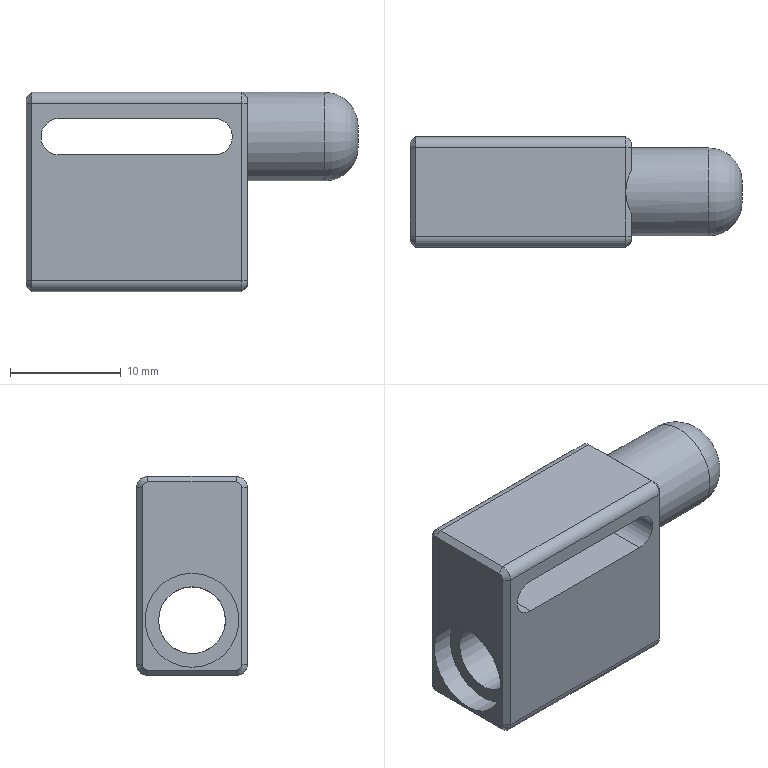Part | NX | 1 solid | 37 faces | box 30 x 10 x 18 mm | volume 2854 mm3 | plane 19 | cylinder 9 | cone 8 | torus 1 | commonest cylinder face diameters 2 x4 3.3 x2 6.05 x1 8 x1 8.5 x1
STEP:
#1=CARTESIAN_POINT('',(5.,9.,3.5));
#2=VERTEX_POINT('',#1);
#3=CARTESIAN_POINT('',(4.5,9.,4.));
#4=VERTEX_POINT('',#3);
#5=CARTESIAN_POINT('',(5.,9.,3.5));
#6=DIRECTION('',(-0.7071,0.,0.7071));
#7=VECTOR('',#6,1000.);
#8=LINE('',#5,#7);
#9=EDGE_CURVE('',#2,#4,#8,.T.);
#10=ORIENTED_EDGE('',*,*,#9,.T.);
#11=CARTESIAN_POINT('',(4.5,5.,4.));
#12=VERTEX_POINT('',#11);
#13=CARTESIAN_POINT('',(4.5,10.,4.));
#14=DIRECTION('',(0.,1.,0.));
#15=VECTOR('',#14,1000.);
#16=LINE('',#13,#15);
#17=EDGE_CURVE('',#12,#4,#16,.T.);
#18=ORIENTED_EDGE('',*,*,#17,.F.);
#19=CARTESIAN_POINT('',(5.,6.936,3.5));
#20=VERTEX_POINT('',#19);
#21=CARTESIAN_POINT('',(8.5,5.,0.));
#22=DIRECTION('',(0.7071,0.,0.7071));
#23=DIRECTION('',(0.7071,0.,-0.7071));
#24=AXIS2_PLACEMENT_3D('',#21,#22,#23);
#25=ELLIPSE('',#24,5.657,4.);
#26=EDGE_CURVE('',#20,#12,#25,.T.);
#27=ORIENTED_EDGE('',*,*,#26,.F.);
#28=CARTESIAN_POINT('',(5.,10.,3.5));
#29=DIRECTION('',(0.,-1.,0.));
#30=VECTOR('',#29,1000.);
#31=LINE('',#28,#30);
#32=EDGE_CURVE('',#2,#20,#31,.T.);
#33=ORIENTED_EDGE('',*,*,#32,.F.);
#34=EDGE_LOOP('',(#10,#18,#27,#33));
#35=FACE_BOUND('',#34,.T.);
#36=CARTESIAN_POINT('',(5.,10.,3.5));
#37=DIRECTION('',(-0.7071,0.,-0.7071));
#38=DIRECTION('',(0.,-1.,0.));
#39=AXIS2_PLACEMENT_3D('',#36,#37,#38);
#40=PLANE('',#39);
#41=ADVANCED_FACE('',(#35),#40,.F.);
#42=CARTESIAN_POINT('',(5.,3.064,3.5));
#43=VERTEX_POINT('',#42);
#44=CARTESIAN_POINT('',(5.,1.,3.5));
#45=VERTEX_POINT('',#44);
#46=CARTESIAN_POINT('',(5.,10.,3.5));
#47=DIRECTION('',(0.,-1.,0.));
#48=VECTOR('',#47,1000.);
#49=LINE('',#46,#48);
#50=EDGE_CURVE('',#43,#45,#49,.T.);
#51=ORIENTED_EDGE('',*,*,#50,.F.);
#52=CARTESIAN_POINT('',(8.5,5.,0.));
#53=DIRECTION('',(0.7071,0.,0.7071));
#54=DIRECTION('',(0.7071,0.,-0.7071));
#55=AXIS2_PLACEMENT_3D('',#52,#53,#54);
#56=ELLIPSE('',#55,5.657,4.);
#57=EDGE_CURVE('',#12,#43,#56,.T.);
#58=ORIENTED_EDGE('',*,*,#57,.F.);
#59=CARTESIAN_POINT('',(4.5,1.,4.));
#60=VERTEX_POINT('',#59);
#61=CARTESIAN_POINT('',(4.5,10.,4.));
#62=DIRECTION('',(0.,1.,0.));
#63=VECTOR('',#62,1000.);
#64=LINE('',#61,#63);
#65=EDGE_CURVE('',#60,#12,#64,.T.);
#66=ORIENTED_EDGE('',*,*,#65,.F.);
#67=CARTESIAN_POINT('',(4.5,1.,4.));
#68=DIRECTION('',(0.7071,0.,-0.7071));
#69=VECTOR('',#68,1000.);
#70=LINE('',#67,#69);
#71=EDGE_CURVE('',#60,#45,#70,.T.);
#72=ORIENTED_EDGE('',*,*,#71,.T.);
#73=EDGE_LOOP('',(#51,#58,#66,#72));
#74=FACE_BOUND('',#73,.T.);
#75=CARTESIAN_POINT('',(5.,10.,3.5));
#76=DIRECTION('',(-0.7071,0.,-0.7071));
#77=DIRECTION('',(0.,-1.,0.));
#78=AXIS2_PLACEMENT_3D('',#75,#76,#77);
#79=PLANE('',#78);
#80=ADVANCED_FACE('',(#74),#79,.F.);
#81=CARTESIAN_POINT('',(5.,9.5,3.));
#82=VERTEX_POINT('',#81);
#83=CARTESIAN_POINT('',(4.5,10.,3.));
#84=VERTEX_POINT('',#83);
#85=CARTESIAN_POINT('',(5.,9.5,3.));
#86=DIRECTION('',(-0.7071,0.7071,0.));
#87=VECTOR('',#86,1000.);
#88=LINE('',#85,#87);
#89=EDGE_CURVE('',#82,#84,#88,.T.);
#90=ORIENTED_EDGE('',*,*,#89,.T.);
#91=CARTESIAN_POINT('',(4.5,9.,3.));
#92=DIRECTION('',(-1.,0.,0.));
#93=DIRECTION('',(0.,0.,1.));
#94=AXIS2_PLACEMENT_3D('',#91,#92,#93);
#95=CIRCLE('',#94,1.);
#96=EDGE_CURVE('',#4,#84,#95,.T.);
#97=ORIENTED_EDGE('',*,*,#96,.F.);
#98=ORIENTED_EDGE('',*,*,#9,.F.);
#99=CARTESIAN_POINT('',(5.,9.,3.));
#100=DIRECTION('',(1.,0.,0.));
#101=DIRECTION('',(0.,-1.,0.));
#102=AXIS2_PLACEMENT_3D('',#99,#100,#101);
#103=CIRCLE('',#102,0.5);
#104=EDGE_CURVE('',#82,#2,#103,.T.);
#105=ORIENTED_EDGE('',*,*,#104,.F.);
#106=EDGE_LOOP('',(#90,#97,#98,#105));
#107=FACE_BOUND('',#106,.T.);
#108=CARTESIAN_POINT('',(5.,9.,3.));
#109=DIRECTION('',(-1.,0.,0.));
#110=DIRECTION('',(0.,0.,1.));
#111=AXIS2_PLACEMENT_3D('',#108,#109,#110);
#112=CONICAL_SURFACE('',#111,0.5,0.7854);
#113=ADVANCED_FACE('',(#107),#112,.T.);
#114=CARTESIAN_POINT('',(4.5,0.,3.));
#115=VERTEX_POINT('',#114);
#116=CARTESIAN_POINT('',(5.,0.5,3.));
#117=VERTEX_POINT('',#116);
#118=CARTESIAN_POINT('',(4.5,0.,3.));
#119=DIRECTION('',(0.7071,0.7071,0.));
#120=VECTOR('',#119,1000.);
#121=LINE('',#118,#120);
#122=EDGE_CURVE('',#115,#117,#121,.T.);
#123=ORIENTED_EDGE('',*,*,#122,.T.);
#124=CARTESIAN_POINT('',(5.,1.,3.));
#125=DIRECTION('',(1.,0.,0.));
#126=DIRECTION('',(0.,-1.,0.));
#127=AXIS2_PLACEMENT_3D('',#124,#125,#126);
#128=CIRCLE('',#127,0.5);
#129=EDGE_CURVE('',#45,#117,#128,.T.);
#130=ORIENTED_EDGE('',*,*,#129,.F.);
#131=ORIENTED_EDGE('',*,*,#71,.F.);
#132=CARTESIAN_POINT('',(4.5,1.,3.));
#133=DIRECTION('',(-1.,0.,0.));
#134=DIRECTION('',(0.,0.,1.));
#135=AXIS2_PLACEMENT_3D('',#132,#133,#134);
#136=CIRCLE('',#135,1.);
#137=EDGE_CURVE('',#115,#60,#136,.T.);
#138=ORIENTED_EDGE('',*,*,#137,.F.);
#139=EDGE_LOOP('',(#123,#130,#131,#138));
#140=FACE_BOUND('',#139,.T.);
#141=CARTESIAN_POINT('',(5.,1.,3.));
#142=DIRECTION('',(-1.,0.,0.));
#143=DIRECTION('',(0.,0.,1.));
#144=AXIS2_PLACEMENT_3D('',#141,#142,#143);
#145=CONICAL_SURFACE('',#144,0.5,0.7854);
#146=ADVANCED_FACE('',(#140),#145,.T.);
#147=CARTESIAN_POINT('',(5.,9.5,-13.));
#148=VERTEX_POINT('',#147);
#149=CARTESIAN_POINT('',(4.5,10.,-13.));
#150=VERTEX_POINT('',#149);
#151=CARTESIAN_POINT('',(5.,9.5,-13.));
#152=DIRECTION('',(-0.7071,0.7071,0.));
#153=VECTOR('',#152,1000.);
#154=LINE('',#151,#153);
#155=EDGE_CURVE('',#148,#150,#154,.T.);
#156=ORIENTED_EDGE('',*,*,#155,.T.);
#157=CARTESIAN_POINT('',(4.5,10.,0.));
#158=DIRECTION('',(0.,0.,-1.));
#159=VECTOR('',#158,1000.);
#160=LINE('',#157,#159);
#161=EDGE_CURVE('',#84,#150,#160,.T.);
#162=ORIENTED_EDGE('',*,*,#161,.F.);
#163=ORIENTED_EDGE('',*,*,#89,.F.);
#164=CARTESIAN_POINT('',(5.,9.5,-14.));
#165=DIRECTION('',(0.,0.,1.));
#166=VECTOR('',#165,1000.);
#167=LINE('',#164,#166);
#168=EDGE_CURVE('',#148,#82,#167,.T.);
#169=ORIENTED_EDGE('',*,*,#168,.F.);
#170=EDGE_LOOP('',(#156,#162,#163,#169));
#171=FACE_BOUND('',#170,.T.);
#172=CARTESIAN_POINT('',(5.,9.5,-14.));
#173=DIRECTION('',(-0.7071,-0.7071,0.));
#174=DIRECTION('',(0.,0.,1.));
#175=AXIS2_PLACEMENT_3D('',#172,#173,#174);
#176=PLANE('',#175);
#177=ADVANCED_FACE('',(#171),#176,.F.);
#178=CARTESIAN_POINT('',(4.5,0.,-13.));
#179=VERTEX_POINT('',#178);
#180=CARTESIAN_POINT('',(5.,0.5,-13.));
#181=VERTEX_POINT('',#180);
#182=CARTESIAN_POINT('',(4.5,0.,-13.));
#183=DIRECTION('',(0.7071,0.7071,0.));
#184=VECTOR('',#183,1000.);
#185=LINE('',#182,#184);
#186=EDGE_CURVE('',#179,#181,#185,.T.);
#187=ORIENTED_EDGE('',*,*,#186,.T.);
#188=CARTESIAN_POINT('',(5.,0.5,-13.));
#189=DIRECTION('',(0.,0.,-1.));
#190=VECTOR('',#189,1000.);
#191=LINE('',#188,#190);
#192=EDGE_CURVE('',#117,#181,#191,.T.);
#193=ORIENTED_EDGE('',*,*,#192,.F.);
#194=ORIENTED_EDGE('',*,*,#122,.F.);
#195=CARTESIAN_POINT('',(4.5,0.,3.));
#196=DIRECTION('',(0.,0.,1.));
#197=VECTOR('',#196,1000.);
#198=LINE('',#195,#197);
#199=EDGE_CURVE('',#179,#115,#198,.T.);
#200=ORIENTED_EDGE('',*,*,#199,.F.);
#201=EDGE_LOOP('',(#187,#193,#194,#200));
#202=FACE_BOUND('',#201,.T.);
#203=CARTESIAN_POINT('',(4.5,0.,0.));
#204=DIRECTION('',(0.7071,-0.7071,0.));
#205=DIRECTION('',(0.,0.,-1.));
#206=AXIS2_PLACEMENT_3D('',#203,#204,#205);
#207=PLANE('',#206);
#208=ADVANCED_FACE('',(#202),#207,.T.);
#209=CARTESIAN_POINT('',(5.,9.,-13.5));
#210=VERTEX_POINT('',#209);
#211=CARTESIAN_POINT('',(4.5,9.,-14.));
#212=VERTEX_POINT('',#211);
#213=CARTESIAN_POINT('',(5.,9.,-13.5));
#214=DIRECTION('',(-0.7071,0.,-0.7071));
#215=VECTOR('',#214,1000.);
#216=LINE('',#213,#215);
#217=EDGE_CURVE('',#210,#212,#216,.T.);
#218=ORIENTED_EDGE('',*,*,#217,.T.);
#219=CARTESIAN_POINT('',(4.5,9.,-13.));
#220=DIRECTION('',(-1.,0.,0.));
#221=DIRECTION('',(0.,0.,1.));
#222=AXIS2_PLACEMENT_3D('',#219,#220,#221);
#223=CIRCLE('',#222,1.);
#224=EDGE_CURVE('',#150,#212,#223,.T.);
#225=ORIENTED_EDGE('',*,*,#224,.F.);
#226=ORIENTED_EDGE('',*,*,#155,.F.);
#227=CARTESIAN_POINT('',(5.,9.,-13.));
#228=DIRECTION('',(1.,0.,0.));
#229=DIRECTION('',(0.,-1.,0.));
#230=AXIS2_PLACEMENT_3D('',#227,#228,#229);
#231=CIRCLE('',#230,0.5);
#232=EDGE_CURVE('',#210,#148,#231,.T.);
#233=ORIENTED_EDGE('',*,*,#232,.F.);
#234=EDGE_LOOP('',(#218,#225,#226,#233));
#235=FACE_BOUND('',#234,.T.);
#236=CARTESIAN_POINT('',(5.,9.,-13.));
#237=DIRECTION('',(-1.,0.,0.));
#238=DIRECTION('',(0.,0.,1.));
#239=AXIS2_PLACEMENT_3D('',#236,#237,#238);
#240=CONICAL_SURFACE('',#239,0.5,0.7854);
#241=ADVANCED_FACE('',(#235),#240,.T.);
#242=CARTESIAN_POINT('',(4.5,1.,-14.));
#243=VERTEX_POINT('',#242);
#244=CARTESIAN_POINT('',(5.,1.,-13.5));
#245=VERTEX_POINT('',#244);
#246=CARTESIAN_POINT('',(4.5,1.,-14.));
#247=DIRECTION('',(0.7071,0.,0.7071));
#248=VECTOR('',#247,1000.);
#249=LINE('',#246,#248);
#250=EDGE_CURVE('',#243,#245,#249,.T.);
#251=ORIENTED_EDGE('',*,*,#250,.T.);
#252=CARTESIAN_POINT('',(5.,1.,-13.));
#253=DIRECTION('',(1.,0.,0.));
#254=DIRECTION('',(0.,-1.,0.));
#255=AXIS2_PLACEMENT_3D('',#252,#253,#254);
#256=CIRCLE('',#255,0.5);
#257=EDGE_CURVE('',#181,#245,#256,.T.);
#258=ORIENTED_EDGE('',*,*,#257,.F.);
#259=ORIENTED_EDGE('',*,*,#186,.F.);
#260=CARTESIAN_POINT('',(4.5,1.,-13.));
#261=DIRECTION('',(-1.,0.,0.));
#262=DIRECTION('',(0.,0.,1.));
#263=AXIS2_PLACEMENT_3D('',#260,#261,#262);
#264=CIRCLE('',#263,1.);
#265=EDGE_CURVE('',#243,#179,#264,.T.);
#266=ORIENTED_EDGE('',*,*,#265,.F.);
#267=EDGE_LOOP('',(#251,#258,#259,#266));
#268=FACE_BOUND('',#267,.T.);
#269=CARTESIAN_POINT('',(5.,1.,-13.));
#270=DIRECTION('',(-1.,0.,0.));
#271=DIRECTION('',(0.,0.,1.));
#272=AXIS2_PLACEMENT_3D('',#269,#270,#271);
#273=CONICAL_SURFACE('',#272,0.5,0.7854);
#274=ADVANCED_FACE('',(#268),#273,.T.);
#275=ORIENTED_EDGE('',*,*,#217,.F.);
#276=CARTESIAN_POINT('',(5.,10.,-13.5));
#277=DIRECTION('',(0.,1.,0.));
#278=VECTOR('',#277,1000.);
#279=LINE('',#276,#278);
#280=EDGE_CURVE('',#245,#210,#279,.T.);
#281=ORIENTED_EDGE('',*,*,#280,.F.);
#282=ORIENTED_EDGE('',*,*,#250,.F.);
#283=CARTESIAN_POINT('',(4.5,0.,-14.));
#284=DIRECTION('',(0.,-1.,0.));
#285=VECTOR('',#284,1000.);
#286=LINE('',#283,#285);
#287=EDGE_CURVE('',#212,#243,#286,.T.);
#288=ORIENTED_EDGE('',*,*,#287,.F.);
#289=EDGE_LOOP('',(#275,#281,#282,#288));
#290=FACE_BOUND('',#289,.T.);
#291=CARTESIAN_POINT('',(4.5,0.,-14.));
#292=DIRECTION('',(-0.7071,0.,0.7071));
#293=DIRECTION('',(0.,-1.,0.));
#294=AXIS2_PLACEMENT_3D('',#291,#292,#293);
#295=PLANE('',#294);
#296=ADVANCED_FACE('',(#290),#295,.F.);
#297=CARTESIAN_POINT('',(-14.5,1.,-14.));
#298=VERTEX_POINT('',#297);
#299=CARTESIAN_POINT('',(-15.,1.,-13.5));
#300=VERTEX_POINT('',#299);
#301=CARTESIAN_POINT('',(-14.5,1.,-14.));
#302=DIRECTION('',(-0.7071,0.,0.7071));
#303=VECTOR('',#302,1000.);
#304=LINE('',#301,#303);
#305=EDGE_CURVE('',#298,#300,#304,.T.);
#306=ORIENTED_EDGE('',*,*,#305,.T.);
#307=CARTESIAN_POINT('',(-15.,9.,-13.5));
#308=VERTEX_POINT('',#307);
#309=CARTESIAN_POINT('',(-15.,10.,-13.5));
#310=DIRECTION('',(0.,-1.,0.));
#311=VECTOR('',#310,1000.);
#312=LINE('',#309,#311);
#313=EDGE_CURVE('',#308,#300,#312,.T.);
#314=ORIENTED_EDGE('',*,*,#313,.F.);
#315=CARTESIAN_POINT('',(-14.5,9.,-14.));
#316=VERTEX_POINT('',#315);
#317=CARTESIAN_POINT('',(-15.,9.,-13.5));
#318=DIRECTION('',(0.7071,0.,-0.7071));
#319=VECTOR('',#318,1000.);
#320=LINE('',#317,#319);
#321=EDGE_CURVE('',#308,#316,#320,.T.);
#322=ORIENTED_EDGE('',*,*,#321,.T.);
#323=CARTESIAN_POINT('',(-14.5,0.,-14.));
#324=DIRECTION('',(0.,1.,0.));
#325=VECTOR('',#324,1000.);
#326=LINE('',#323,#325);
#327=EDGE_CURVE('',#298,#316,#326,.T.);
#328=ORIENTED_EDGE('',*,*,#327,.F.);
#329=EDGE_LOOP('',(#306,#314,#322,#328));
#330=FACE_BOUND('',#329,.T.);
#331=CARTESIAN_POINT('',(-14.5,0.,-14.));
#332=DIRECTION('',(0.7071,0.,0.7071));
#333=DIRECTION('',(0.,1.,0.));
#334=AXIS2_PLACEMENT_3D('',#331,#332,#333);
#335=PLANE('',#334);
#336=ADVANCED_FACE('',(#330),#335,.F.);
#337=CARTESIAN_POINT('',(-15.,9.5,-13.));
#338=VERTEX_POINT('',#337);
#339=CARTESIAN_POINT('',(-14.5,10.,-13.));
#340=VERTEX_POINT('',#339);
#341=CARTESIAN_POINT('',(-15.,9.5,-13.));
#342=DIRECTION('',(0.7071,0.7071,0.));
#343=VECTOR('',#342,1000.);
#344=LINE('',#341,#343);
#345=EDGE_CURVE('',#338,#340,#344,.T.);
#346=ORIENTED_EDGE('',*,*,#345,.T.);
#347=CARTESIAN_POINT('',(-14.5,9.,-13.));
#348=DIRECTION('',(1.,0.,0.));
#349=DIRECTION('',(0.,0.,-1.));
#350=AXIS2_PLACEMENT_3D('',#347,#348,#349);
#351=CIRCLE('',#350,1.);
#352=EDGE_CURVE('',#316,#340,#351,.T.);
#353=ORIENTED_EDGE('',*,*,#352,.F.);
#354=ORIENTED_EDGE('',*,*,#321,.F.);
#355=CARTESIAN_POINT('',(-15.,9.,-13.));
#356=DIRECTION('',(-1.,0.,0.));
#357=DIRECTION('',(0.,0.,-1.));
#358=AXIS2_PLACEMENT_3D('',#355,#356,#357);
#359=CIRCLE('',#358,0.5);
#360=EDGE_CURVE('',#338,#308,#359,.T.);
#361=ORIENTED_EDGE('',*,*,#360,.F.);
#362=EDGE_LOOP('',(#346,#353,#354,#361));
#363=FACE_BOUND('',#362,.T.);
#364=CARTESIAN_POINT('',(-15.,9.,-13.));
#365=DIRECTION('',(1.,0.,0.));
#366=DIRECTION('',(0.,0.,-1.));
#367=AXIS2_PLACEMENT_3D('',#364,#365,#366);
#368=CONICAL_SURFACE('',#367,0.5,0.7854);
#369=ADVANCED_FACE('',(#363),#368,.T.);
#370=CARTESIAN_POINT('',(-14.5,0.,-13.));
#371=VERTEX_POINT('',#370);
#372=CARTESIAN_POINT('',(-15.,0.5,-13.));
#373=VERTEX_POINT('',#372);
#374=CARTESIAN_POINT('',(-14.5,0.,-13.));
#375=DIRECTION('',(-0.7071,0.7071,0.));
#376=VECTOR('',#375,1000.);
#377=LINE('',#374,#376);
#378=EDGE_CURVE('',#371,#373,#377,.T.);
#379=ORIENTED_EDGE('',*,*,#378,.T.);
#380=CARTESIAN_POINT('',(-15.,1.,-13.));
#381=DIRECTION('',(-1.,0.,0.));
#382=DIRECTION('',(0.,0.,-1.));
#383=AXIS2_PLACEMENT_3D('',#380,#381,#382);
#384=CIRCLE('',#383,0.5);
#385=EDGE_CURVE('',#300,#373,#384,.T.);
#386=ORIENTED_EDGE('',*,*,#385,.F.);
#387=ORIENTED_EDGE('',*,*,#305,.F.);
#388=CARTESIAN_POINT('',(-14.5,1.,-13.));
#389=DIRECTION('',(1.,0.,0.));
#390=DIRECTION('',(0.,0.,-1.));
#391=AXIS2_PLACEMENT_3D('',#388,#389,#390);
#392=CIRCLE('',#391,1.);
#393=EDGE_CURVE('',#371,#298,#392,.T.);
#394=ORIENTED_EDGE('',*,*,#393,.F.);
#395=EDGE_LOOP('',(#379,#386,#387,#394));
#396=FACE_BOUND('',#395,.T.);
#397=CARTESIAN_POINT('',(-15.,1.,-13.));
#398=DIRECTION('',(1.,0.,0.));
#399=DIRECTION('',(0.,0.,-1.));
#400=AXIS2_PLACEMENT_3D('',#397,#398,#399);
#401=CONICAL_SURFACE('',#400,0.5,0.7854);
#402=ADVANCED_FACE('',(#396),#401,.T.);
#403=CARTESIAN_POINT('',(-15.,9.5,3.));
#404=VERTEX_POINT('',#403);
#405=CARTESIAN_POINT('',(-14.5,10.,3.));
#406=VERTEX_POINT('',#405);
#407=CARTESIAN_POINT('',(-15.,9.5,3.));
#408=DIRECTION('',(0.7071,0.7071,0.));
#409=VECTOR('',#408,1000.);
#410=LINE('',#407,#409);
#411=EDGE_CURVE('',#404,#406,#410,.T.);
#412=ORIENTED_EDGE('',*,*,#411,.T.);
#413=CARTESIAN_POINT('',(-14.5,10.,0.));
#414=DIRECTION('',(0.,0.,1.));
#415=VECTOR('',#414,1000.);
#416=LINE('',#413,#415);
#417=EDGE_CURVE('',#340,#406,#416,.T.);
#418=ORIENTED_EDGE('',*,*,#417,.F.);
#419=ORIENTED_EDGE('',*,*,#345,.F.);
#420=CARTESIAN_POINT('',(-15.,9.5,4.));
#421=DIRECTION('',(0.,0.,-1.));
#422=VECTOR('',#421,1000.);
#423=LINE('',#420,#422);
#424=EDGE_CURVE('',#404,#338,#423,.T.);
#425=ORIENTED_EDGE('',*,*,#424,.F.);
#426=EDGE_LOOP('',(#412,#418,#419,#425));
#427=FACE_BOUND('',#426,.T.);
#428=CARTESIAN_POINT('',(-14.5,10.,0.));
#429=DIRECTION('',(0.7071,-0.7071,0.));
#430=DIRECTION('',(0.,0.,1.));
#431=AXIS2_PLACEMENT_3D('',#428,#429,#430);
#432=PLANE('',#431);
#433=ADVANCED_FACE('',(#427),#432,.F.);
#434=CARTESIAN_POINT('',(-14.5,0.,3.));
#435=VERTEX_POINT('',#434);
#436=CARTESIAN_POINT('',(-15.,0.5,3.));
#437=VERTEX_POINT('',#436);
#438=CARTESIAN_POINT('',(-14.5,0.,3.));
#439=DIRECTION('',(-0.7071,0.7071,0.));
#440=VECTOR('',#439,1000.);
#441=LINE('',#438,#440);
#442=EDGE_CURVE('',#435,#437,#441,.T.);
#443=ORIENTED_EDGE('',*,*,#442,.T.);
#444=CARTESIAN_POINT('',(-15.,0.5,3.));
#445=DIRECTION('',(0.,0.,1.));
#446=VECTOR('',#445,1000.);
#447=LINE('',#444,#446);
#448=EDGE_CURVE('',#373,#437,#447,.T.);
#449=ORIENTED_EDGE('',*,*,#448,.F.);
#450=ORIENTED_EDGE('',*,*,#378,.F.);
#451=CARTESIAN_POINT('',(-14.5,0.,-13.));
#452=DIRECTION('',(0.,0.,-1.));
#453=VECTOR('',#452,1000.);
#454=LINE('',#451,#453);
#455=EDGE_CURVE('',#435,#371,#454,.T.);
#456=ORIENTED_EDGE('',*,*,#455,.F.);
#457=EDGE_LOOP('',(#443,#449,#450,#456));
#458=FACE_BOUND('',#457,.T.);
#459=CARTESIAN_POINT('',(-15.,0.5,4.));
#460=DIRECTION('',(-0.7071,-0.7071,0.));
#461=DIRECTION('',(0.,0.,-1.));
#462=AXIS2_PLACEMENT_3D('',#459,#460,#461);
#463=PLANE('',#462);
#464=ADVANCED_FACE('',(#458),#463,.T.);
#465=CARTESIAN_POINT('',(-15.,9.,3.5));
#466=VERTEX_POINT('',#465);
#467=CARTESIAN_POINT('',(-14.5,9.,4.));
#468=VERTEX_POINT('',#467);
#469=CARTESIAN_POINT('',(-15.,9.,3.5));
#470=DIRECTION('',(0.7071,0.,0.7071));
#471=VECTOR('',#470,1000.);
#472=LINE('',#469,#471);
#473=EDGE_CURVE('',#466,#468,#472,.T.);
#474=ORIENTED_EDGE('',*,*,#473,.T.);
#475=CARTESIAN_POINT('',(-14.5,9.,3.));
#476=DIRECTION('',(1.,0.,0.));
#477=DIRECTION('',(0.,0.,-1.));
#478=AXIS2_PLACEMENT_3D('',#475,#476,#477);
#479=CIRCLE('',#478,1.);
#480=EDGE_CURVE('',#406,#468,#479,.T.);
#481=ORIENTED_EDGE('',*,*,#480,.F.);
#482=ORIENTED_EDGE('',*,*,#411,.F.);
#483=CARTESIAN_POINT('',(-15.,9.,3.));
#484=DIRECTION('',(-1.,0.,0.));
#485=DIRECTION('',(0.,0.,-1.));
#486=AXIS2_PLACEMENT_3D('',#483,#484,#485);
#487=CIRCLE('',#486,0.5);
#488=EDGE_CURVE('',#466,#404,#487,.T.);
#489=ORIENTED_EDGE('',*,*,#488,.F.);
#490=EDGE_LOOP('',(#474,#481,#482,#489));
#491=FACE_BOUND('',#490,.T.);
#492=CARTESIAN_POINT('',(-15.,9.,3.));
#493=DIRECTION('',(1.,0.,0.));
#494=DIRECTION('',(0.,0.,-1.));
#495=AXIS2_PLACEMENT_3D('',#492,#493,#494);
#496=CONICAL_SURFACE('',#495,0.5,0.7854);
#497=ADVANCED_FACE('',(#491),#496,.T.);
#498=CARTESIAN_POINT('',(-14.5,1.,4.));
#499=VERTEX_POINT('',#498);
#500=CARTESIAN_POINT('',(-15.,1.,3.5));
#501=VERTEX_POINT('',#500);
#502=CARTESIAN_POINT('',(-14.5,1.,4.));
#503=DIRECTION('',(-0.7071,0.,-0.7071));
#504=VECTOR('',#503,1000.);
#505=LINE('',#502,#504);
#506=EDGE_CURVE('',#499,#501,#505,.T.);
#507=ORIENTED_EDGE('',*,*,#506,.T.);
#508=CARTESIAN_POINT('',(-15.,1.,3.));
#509=DIRECTION('',(-1.,0.,0.));
#510=DIRECTION('',(0.,0.,-1.));
#511=AXIS2_PLACEMENT_3D('',#508,#509,#510);
#512=CIRCLE('',#511,0.5);
#513=EDGE_CURVE('',#437,#501,#512,.T.);
#514=ORIENTED_EDGE('',*,*,#513,.F.);
#515=ORIENTED_EDGE('',*,*,#442,.F.);
#516=CARTESIAN_POINT('',(-14.5,1.,3.));
#517=DIRECTION('',(1.,0.,0.));
#518=DIRECTION('',(0.,0.,-1.));
#519=AXIS2_PLACEMENT_3D('',#516,#517,#518);
#520=CIRCLE('',#519,1.);
#521=EDGE_CURVE('',#499,#435,#520,.T.);
#522=ORIENTED_EDGE('',*,*,#521,.F.);
#523=EDGE_LOOP('',(#507,#514,#515,#522));
#524=FACE_BOUND('',#523,.T.);
#525=CARTESIAN_POINT('',(-15.,1.,3.));
#526=DIRECTION('',(1.,0.,0.));
#527=DIRECTION('',(0.,0.,-1.));
#528=AXIS2_PLACEMENT_3D('',#525,#526,#527);
#529=CONICAL_SURFACE('',#528,0.5,0.7854);
#530=ADVANCED_FACE('',(#524),#529,.T.);
#531=ORIENTED_EDGE('',*,*,#473,.F.);
#532=CARTESIAN_POINT('',(-15.,10.,3.5));
#533=DIRECTION('',(0.,1.,0.));
#534=VECTOR('',#533,1000.);
#535=LINE('',#532,#534);
#536=EDGE_CURVE('',#501,#466,#535,.T.);
#537=ORIENTED_EDGE('',*,*,#536,.F.);
#538=ORIENTED_EDGE('',*,*,#506,.F.);
#539=CARTESIAN_POINT('',(-14.5,10.,4.));
#540=DIRECTION('',(0.,-1.,0.));
#541=VECTOR('',#540,1000.);
#542=LINE('',#539,#541);
#543=EDGE_CURVE('',#468,#499,#542,.T.);
#544=ORIENTED_EDGE('',*,*,#543,.F.);
#545=EDGE_LOOP('',(#531,#537,#538,#544));
#546=FACE_BOUND('',#545,.T.);
#547=CARTESIAN_POINT('',(-14.5,10.,4.));
#548=DIRECTION('',(0.7071,0.,-0.7071));
#549=DIRECTION('',(0.,-1.,0.));
#550=AXIS2_PLACEMENT_3D('',#547,#548,#549);
#551=PLANE('',#550);
#552=ADVANCED_FACE('',(#546),#551,.F.);
#553=CARTESIAN_POINT('',(-13.,5.,-5.975));
#554=VERTEX_POINT('',#553);
#555=CARTESIAN_POINT('',(-13.,5.,-9.));
#556=DIRECTION('',(1.,0.,0.));
#557=DIRECTION('',(0.,0.,1.));
#558=AXIS2_PLACEMENT_3D('',#555,#556,#557);
#559=CIRCLE('',#558,3.025);
#560=EDGE_CURVE('',#554,#554,#559,.T.);
#561=ORIENTED_EDGE('',*,*,#560,.T.);
#562=EDGE_LOOP('',(#561));
#563=FACE_BOUND('',#562,.T.);
#564=CARTESIAN_POINT('',(-13.,5.,-4.75));
#565=VERTEX_POINT('',#564);
#566=CARTESIAN_POINT('',(-13.,5.,-9.));
#567=DIRECTION('',(-1.,0.,0.));
#568=DIRECTION('',(0.,0.,1.));
#569=AXIS2_PLACEMENT_3D('',#566,#567,#568);
#570=CIRCLE('',#569,4.25);
#571=EDGE_CURVE('',#565,#565,#570,.T.);
#572=ORIENTED_EDGE('',*,*,#571,.T.);
#573=EDGE_LOOP('',(#572));
#574=FACE_BOUND('',#573,.T.);
#575=CARTESIAN_POINT('',(-13.,5.,-9.));
#576=DIRECTION('',(-1.,0.,0.));
#577=DIRECTION('',(0.,0.,1.));
#578=AXIS2_PLACEMENT_3D('',#575,#576,#577);
#579=PLANE('',#578);
#580=ADVANCED_FACE('',(#563,#574),#579,.T.);
#581=CARTESIAN_POINT('',(5.,1.,4.));
#582=DIRECTION('',(1.,0.,0.));
#583=VECTOR('',#582,1000.);
#584=LINE('',#581,#583);
#585=EDGE_CURVE('',#499,#60,#584,.T.);
#586=ORIENTED_EDGE('',*,*,#585,.F.);
#587=ORIENTED_EDGE('',*,*,#521,.T.);
#588=CARTESIAN_POINT('',(-15.,0.,3.));
#589=DIRECTION('',(-1.,0.,0.));
#590=VECTOR('',#589,1000.);
#591=LINE('',#588,#590);
#592=EDGE_CURVE('',#115,#435,#591,.T.);
#593=ORIENTED_EDGE('',*,*,#592,.F.);
#594=ORIENTED_EDGE('',*,*,#137,.T.);
#595=EDGE_LOOP('',(#586,#587,#593,#594));
#596=FACE_BOUND('',#595,.T.);
#597=CARTESIAN_POINT('',(-15.,1.,3.));
#598=DIRECTION('',(-1.,0.,0.));
#599=DIRECTION('',(0.,0.,1.));
#600=AXIS2_PLACEMENT_3D('',#597,#598,#599);
#601=CYLINDRICAL_SURFACE('',#600,1.);
#602=ADVANCED_FACE('',(#596),#601,.T.);
#603=CARTESIAN_POINT('',(0.,10.,3.));
#604=DIRECTION('',(1.,0.,0.));
#605=VECTOR('',#604,1000.);
#606=LINE('',#603,#605);
#607=EDGE_CURVE('',#406,#84,#606,.T.);
#608=ORIENTED_EDGE('',*,*,#607,.F.);
#609=ORIENTED_EDGE('',*,*,#480,.T.);
#610=CARTESIAN_POINT('',(-15.,9.,4.));
#611=DIRECTION('',(-1.,0.,0.));
#612=VECTOR('',#611,1000.);
#613=LINE('',#610,#612);
#614=EDGE_CURVE('',#4,#468,#613,.T.);
#615=ORIENTED_EDGE('',*,*,#614,.F.);
#616=ORIENTED_EDGE('',*,*,#96,.T.);
#617=EDGE_LOOP('',(#608,#609,#615,#616));
#618=FACE_BOUND('',#617,.T.);
#619=CARTESIAN_POINT('',(0.,9.,3.));
#620=DIRECTION('',(1.,0.,0.));
#621=DIRECTION('',(0.,0.,-1.));
#622=AXIS2_PLACEMENT_3D('',#619,#620,#621);
#623=CYLINDRICAL_SURFACE('',#622,1.);
#624=ADVANCED_FACE('',(#618),#623,.T.);
#625=CARTESIAN_POINT('',(5.,0.,-13.));
#626=DIRECTION('',(1.,0.,0.));
#627=VECTOR('',#626,1000.);
#628=LINE('',#625,#627);
#629=EDGE_CURVE('',#371,#179,#628,.T.);
#630=ORIENTED_EDGE('',*,*,#629,.F.);
#631=ORIENTED_EDGE('',*,*,#393,.T.);
#632=CARTESIAN_POINT('',(-15.,1.,-14.));
#633=DIRECTION('',(-1.,0.,0.));
#634=VECTOR('',#633,1000.);
#635=LINE('',#632,#634);
#636=EDGE_CURVE('',#243,#298,#635,.T.);
#637=ORIENTED_EDGE('',*,*,#636,.F.);
#638=ORIENTED_EDGE('',*,*,#265,.T.);
#639=EDGE_LOOP('',(#630,#631,#637,#638));
#640=FACE_BOUND('',#639,.T.);
#641=CARTESIAN_POINT('',(0.,1.,-13.));
#642=DIRECTION('',(1.,0.,0.));
#643=DIRECTION('',(0.,0.,-1.));
#644=AXIS2_PLACEMENT_3D('',#641,#642,#643);
#645=CYLINDRICAL_SURFACE('',#644,1.);
#646=ADVANCED_FACE('',(#640),#645,.T.);
#647=CARTESIAN_POINT('',(0.,9.,-14.));
#648=DIRECTION('',(1.,0.,0.));
#649=VECTOR('',#648,1000.);
#650=LINE('',#647,#649);
#651=EDGE_CURVE('',#316,#212,#650,.T.);
#652=ORIENTED_EDGE('',*,*,#651,.F.);
#653=ORIENTED_EDGE('',*,*,#352,.T.);
#654=CARTESIAN_POINT('',(0.,10.,-13.));
#655=DIRECTION('',(-1.,0.,0.));
#656=VECTOR('',#655,1000.);
#657=LINE('',#654,#656);
#658=EDGE_CURVE('',#150,#340,#657,.T.);
#659=ORIENTED_EDGE('',*,*,#658,.F.);
#660=ORIENTED_EDGE('',*,*,#224,.T.);
#661=EDGE_LOOP('',(#652,#653,#659,#660));
#662=FACE_BOUND('',#661,.T.);
#663=CARTESIAN_POINT('',(0.,9.,-13.));
#664=DIRECTION('',(1.,0.,0.));
#665=DIRECTION('',(0.,0.,-1.));
#666=AXIS2_PLACEMENT_3D('',#663,#664,#665);
#667=CYLINDRICAL_SURFACE('',#666,1.);
#668=ADVANCED_FACE('',(#662),#667,.T.);
#669=ORIENTED_EDGE('',*,*,#636,.T.);
#670=ORIENTED_EDGE('',*,*,#327,.T.);
#671=ORIENTED_EDGE('',*,*,#651,.T.);
#672=ORIENTED_EDGE('',*,*,#287,.T.);
#673=EDGE_LOOP('',(#669,#670,#671,#672));
#674=FACE_BOUND('',#673,.T.);
#675=CARTESIAN_POINT('',(0.,0.,-14.));
#676=DIRECTION('',(0.,0.,1.));
#677=DIRECTION('',(1.,0.,0.));
#678=AXIS2_PLACEMENT_3D('',#675,#676,#677);
#679=PLANE('',#678);
#680=ADVANCED_FACE('',(#674),#679,.F.);
#681=ORIENTED_EDGE('',*,*,#104,.T.);
#682=ORIENTED_EDGE('',*,*,#32,.T.);
#683=CARTESIAN_POINT('',(5.,5.,0.));
#684=DIRECTION('',(1.,0.,0.));
#685=DIRECTION('',(0.,-1.,0.));
#686=AXIS2_PLACEMENT_3D('',#683,#684,#685);
#687=CIRCLE('',#686,4.);
#688=EDGE_CURVE('',#43,#20,#687,.T.);
#689=ORIENTED_EDGE('',*,*,#688,.F.);
#690=ORIENTED_EDGE('',*,*,#50,.T.);
#691=ORIENTED_EDGE('',*,*,#129,.T.);
#692=ORIENTED_EDGE('',*,*,#192,.T.);
#693=ORIENTED_EDGE('',*,*,#257,.T.);
#694=ORIENTED_EDGE('',*,*,#280,.T.);
#695=ORIENTED_EDGE('',*,*,#232,.T.);
#696=ORIENTED_EDGE('',*,*,#168,.T.);
#697=EDGE_LOOP('',(#681,#682,#689,#690,#691,#692,#693,#694,#695,#696));
#698=FACE_BOUND('',#697,.T.);
#699=CARTESIAN_POINT('',(5.,8.025,-9.));
#700=VERTEX_POINT('',#699);
#701=CARTESIAN_POINT('',(5.,5.,-9.));
#702=DIRECTION('',(1.,0.,0.));
#703=DIRECTION('',(0.,1.,0.));
#704=AXIS2_PLACEMENT_3D('',#701,#702,#703);
#705=CIRCLE('',#704,3.025);
#706=EDGE_CURVE('',#700,#700,#705,.T.);
#707=ORIENTED_EDGE('',*,*,#706,.F.);
#708=EDGE_LOOP('',(#707));
#709=FACE_BOUND('',#708,.T.);
#710=CARTESIAN_POINT('',(5.,10.,-14.));
#711=DIRECTION('',(-1.,0.,0.));
#712=DIRECTION('',(0.,-1.,0.));
#713=AXIS2_PLACEMENT_3D('',#710,#711,#712);
#714=PLANE('',#713);
#715=ADVANCED_FACE('',(#698,#709),#714,.F.);
#716=CARTESIAN_POINT('',(2.,0.,1.65));
#717=VERTEX_POINT('',#716);
#718=CARTESIAN_POINT('',(-12.,0.,1.65));
#719=VERTEX_POINT('',#718);
#720=CARTESIAN_POINT('',(0.,0.,1.65));
#721=DIRECTION('',(-1.,0.,0.));
#722=VECTOR('',#721,1000.);
#723=LINE('',#720,#722);
#724=EDGE_CURVE('',#717,#719,#723,.T.);
#725=ORIENTED_EDGE('',*,*,#724,.T.);
#726=CARTESIAN_POINT('',(-12.,10.,1.65));
#727=VERTEX_POINT('',#726);
#728=CARTESIAN_POINT('',(-12.,-101.,1.65));
#729=DIRECTION('',(0.,1.,0.));
#730=VECTOR('',#729,1000.);
#731=LINE('',#728,#730);
#732=EDGE_CURVE('',#719,#727,#731,.T.);
#733=ORIENTED_EDGE('',*,*,#732,.T.);
#734=CARTESIAN_POINT('',(2.,10.,1.65));
#735=VERTEX_POINT('',#734);
#736=CARTESIAN_POINT('',(-12.,10.,1.65));
#737=DIRECTION('',(1.,0.,0.));
#738=VECTOR('',#737,1000.);
#739=LINE('',#736,#738);
#740=EDGE_CURVE('',#727,#735,#739,.T.);
#741=ORIENTED_EDGE('',*,*,#740,.T.);
#742=CARTESIAN_POINT('',(2.,-101.,1.65));
#743=DIRECTION('',(0.,1.,0.));
#744=VECTOR('',#743,1000.);
#745=LINE('',#742,#744);
#746=EDGE_CURVE('',#717,#735,#745,.T.);
#747=ORIENTED_EDGE('',*,*,#746,.F.);
#748=EDGE_LOOP('',(#725,#733,#741,#747));
#749=FACE_BOUND('',#748,.T.);
#750=CARTESIAN_POINT('',(-12.,-101.,1.65));
#751=DIRECTION('',(0.,0.,1.));
#752=DIRECTION('',(1.,0.,0.));
#753=AXIS2_PLACEMENT_3D('',#750,#751,#752);
#754=PLANE('',#753);
#755=ADVANCED_FACE('',(#749),#754,.F.);
#756=CARTESIAN_POINT('',(2.,0.,-1.65));
#757=VERTEX_POINT('',#756);
#758=CARTESIAN_POINT('',(2.,0.,0.));
#759=DIRECTION('',(0.,-1.,0.));
#760=DIRECTION('',(0.,0.,-1.));
#761=AXIS2_PLACEMENT_3D('',#758,#759,#760);
#762=CIRCLE('',#761,1.65);
#763=EDGE_CURVE('',#757,#717,#762,.T.);
#764=ORIENTED_EDGE('',*,*,#763,.T.);
#765=ORIENTED_EDGE('',*,*,#746,.T.);
#766=CARTESIAN_POINT('',(2.,10.,-1.65));
#767=VERTEX_POINT('',#766);
#768=CARTESIAN_POINT('',(2.,10.,0.));
#769=DIRECTION('',(0.,1.,0.));
#770=DIRECTION('',(0.,0.,1.));
#771=AXIS2_PLACEMENT_3D('',#768,#769,#770);
#772=CIRCLE('',#771,1.65);
#773=EDGE_CURVE('',#735,#767,#772,.T.);
#774=ORIENTED_EDGE('',*,*,#773,.T.);
#775=CARTESIAN_POINT('',(2.,-101.,-1.65));
#776=DIRECTION('',(0.,1.,0.));
#777=VECTOR('',#776,1000.);
#778=LINE('',#775,#777);
#779=EDGE_CURVE('',#757,#767,#778,.T.);
#780=ORIENTED_EDGE('',*,*,#779,.F.);
#781=EDGE_LOOP('',(#764,#765,#774,#780));
#782=FACE_BOUND('',#781,.T.);
#783=CARTESIAN_POINT('',(2.,-101.,0.));
#784=DIRECTION('',(0.,1.,0.));
#785=DIRECTION('',(0.,0.,1.));
#786=AXIS2_PLACEMENT_3D('',#783,#784,#785);
#787=CYLINDRICAL_SURFACE('',#786,1.65);
#788=ADVANCED_FACE('',(#782),#787,.F.);
#789=CARTESIAN_POINT('',(-12.,0.,-1.65));
#790=VERTEX_POINT('',#789);
#791=CARTESIAN_POINT('',(0.,0.,-1.65));
#792=DIRECTION('',(1.,0.,0.));
#793=VECTOR('',#792,1000.);
#794=LINE('',#791,#793);
#795=EDGE_CURVE('',#790,#757,#794,.T.);
#796=ORIENTED_EDGE('',*,*,#795,.T.);
#797=ORIENTED_EDGE('',*,*,#779,.T.);
#798=CARTESIAN_POINT('',(-12.,10.,-1.65));
#799=VERTEX_POINT('',#798);
#800=CARTESIAN_POINT('',(-12.,10.,-1.65));
#801=DIRECTION('',(-1.,0.,0.));
#802=VECTOR('',#801,1000.);
#803=LINE('',#800,#802);
#804=EDGE_CURVE('',#767,#799,#803,.T.);
#805=ORIENTED_EDGE('',*,*,#804,.T.);
#806=CARTESIAN_POINT('',(-12.,-101.,-1.65));
#807=DIRECTION('',(0.,1.,0.));
#808=VECTOR('',#807,1000.);
#809=LINE('',#806,#808);
#810=EDGE_CURVE('',#790,#799,#809,.T.);
#811=ORIENTED_EDGE('',*,*,#810,.F.);
#812=EDGE_LOOP('',(#796,#797,#805,#811));
#813=FACE_BOUND('',#812,.T.);
#814=CARTESIAN_POINT('',(-12.,-101.,-1.65));
#815=DIRECTION('',(0.,0.,-1.));
#816=DIRECTION('',(-1.,0.,0.));
#817=AXIS2_PLACEMENT_3D('',#814,#815,#816);
#818=PLANE('',#817);
#819=ADVANCED_FACE('',(#813),#818,.F.);
#820=CARTESIAN_POINT('',(-12.,0.,0.));
#821=DIRECTION('',(0.,-1.,0.));
#822=DIRECTION('',(0.,0.,-1.));
#823=AXIS2_PLACEMENT_3D('',#820,#821,#822);
#824=CIRCLE('',#823,1.65);
#825=EDGE_CURVE('',#719,#790,#824,.T.);
#826=ORIENTED_EDGE('',*,*,#825,.T.);
#827=ORIENTED_EDGE('',*,*,#810,.T.);
#828=CARTESIAN_POINT('',(-12.,10.,0.));
#829=DIRECTION('',(0.,1.,0.));
#830=DIRECTION('',(0.,0.,1.));
#831=AXIS2_PLACEMENT_3D('',#828,#829,#830);
#832=CIRCLE('',#831,1.65);
#833=EDGE_CURVE('',#799,#727,#832,.T.);
#834=ORIENTED_EDGE('',*,*,#833,.T.);
#835=ORIENTED_EDGE('',*,*,#732,.F.);
#836=EDGE_LOOP('',(#826,#827,#834,#835));
#837=FACE_BOUND('',#836,.T.);
#838=CARTESIAN_POINT('',(-12.,-101.,0.));
#839=DIRECTION('',(0.,1.,0.));
#840=DIRECTION('',(0.,0.,1.));
#841=AXIS2_PLACEMENT_3D('',#838,#839,#840);
#842=CYLINDRICAL_SURFACE('',#841,1.65);
#843=ADVANCED_FACE('',(#837),#842,.F.);
#844=ORIENTED_EDGE('',*,*,#825,.F.);
#845=ORIENTED_EDGE('',*,*,#724,.F.);
#846=ORIENTED_EDGE('',*,*,#763,.F.);
#847=ORIENTED_EDGE('',*,*,#795,.F.);
#848=EDGE_LOOP('',(#844,#845,#846,#847));
#849=FACE_BOUND('',#848,.T.);
#850=ORIENTED_EDGE('',*,*,#592,.T.);
#851=ORIENTED_EDGE('',*,*,#455,.T.);
#852=ORIENTED_EDGE('',*,*,#629,.T.);
#853=ORIENTED_EDGE('',*,*,#199,.T.);
#854=EDGE_LOOP('',(#850,#851,#852,#853));
#855=FACE_BOUND('',#854,.T.);
#856=CARTESIAN_POINT('',(0.,0.,0.));
#857=DIRECTION('',(0.,-1.,0.));
#858=DIRECTION('',(0.,0.,-1.));
#859=AXIS2_PLACEMENT_3D('',#856,#857,#858);
#860=PLANE('',#859);
#861=ADVANCED_FACE('',(#849,#855),#860,.T.);
#862=ORIENTED_EDGE('',*,*,#658,.T.);
#863=ORIENTED_EDGE('',*,*,#417,.T.);
#864=ORIENTED_EDGE('',*,*,#607,.T.);
#865=ORIENTED_EDGE('',*,*,#161,.T.);
#866=EDGE_LOOP('',(#862,#863,#864,#865));
#867=FACE_BOUND('',#866,.T.);
#868=ORIENTED_EDGE('',*,*,#740,.F.);
#869=ORIENTED_EDGE('',*,*,#833,.F.);
#870=ORIENTED_EDGE('',*,*,#804,.F.);
#871=ORIENTED_EDGE('',*,*,#773,.F.);
#872=EDGE_LOOP('',(#868,#869,#870,#871));
#873=FACE_BOUND('',#872,.T.);
#874=CARTESIAN_POINT('',(0.,10.,0.));
#875=DIRECTION('',(0.,-1.,0.));
#876=DIRECTION('',(0.,0.,-1.));
#877=AXIS2_PLACEMENT_3D('',#874,#875,#876);
#878=PLANE('',#877);
#879=ADVANCED_FACE('',(#867,#873),#878,.F.);
#880=ORIENTED_EDGE('',*,*,#614,.T.);
#881=ORIENTED_EDGE('',*,*,#543,.T.);
#882=ORIENTED_EDGE('',*,*,#585,.T.);
#883=ORIENTED_EDGE('',*,*,#65,.T.);
#884=ORIENTED_EDGE('',*,*,#17,.T.);
#885=EDGE_LOOP('',(#880,#881,#882,#883,#884));
#886=FACE_BOUND('',#885,.T.);
#887=CARTESIAN_POINT('',(-15.,10.,4.));
#888=DIRECTION('',(0.,0.,-1.));
#889=DIRECTION('',(-1.,0.,0.));
#890=AXIS2_PLACEMENT_3D('',#887,#888,#889);
#891=PLANE('',#890);
#892=ADVANCED_FACE('',(#886),#891,.F.);
#893=CARTESIAN_POINT('',(-15.,5.,-4.75));
#894=VERTEX_POINT('',#893);
#895=CARTESIAN_POINT('',(-15.,5.,-9.));
#896=DIRECTION('',(-1.,0.,0.));
#897=DIRECTION('',(0.,0.,1.));
#898=AXIS2_PLACEMENT_3D('',#895,#896,#897);
#899=CIRCLE('',#898,4.25);
#900=EDGE_CURVE('',#894,#894,#899,.T.);
#901=ORIENTED_EDGE('',*,*,#900,.F.);
#902=EDGE_LOOP('',(#901));
#903=FACE_BOUND('',#902,.T.);
#904=ORIENTED_EDGE('',*,*,#360,.T.);
#905=ORIENTED_EDGE('',*,*,#313,.T.);
#906=ORIENTED_EDGE('',*,*,#385,.T.);
#907=ORIENTED_EDGE('',*,*,#448,.T.);
#908=ORIENTED_EDGE('',*,*,#513,.T.);
#909=ORIENTED_EDGE('',*,*,#536,.T.);
#910=ORIENTED_EDGE('',*,*,#488,.T.);
#911=ORIENTED_EDGE('',*,*,#424,.T.);
#912=EDGE_LOOP('',(#904,#905,#906,#907,#908,#909,#910,#911));
#913=FACE_BOUND('',#912,.T.);
#914=CARTESIAN_POINT('',(-15.,10.,4.));
#915=DIRECTION('',(1.,0.,0.));
#916=DIRECTION('',(0.,0.,-1.));
#917=AXIS2_PLACEMENT_3D('',#914,#915,#916);
#918=PLANE('',#917);
#919=ADVANCED_FACE('',(#903,#913),#918,.F.);
#920=CARTESIAN_POINT('',(15.,5.,1.));
#921=VERTEX_POINT('',#920);
#922=CARTESIAN_POINT('',(15.,5.,0.));
#923=DIRECTION('',(1.,0.,0.));
#924=DIRECTION('',(0.,0.,1.));
#925=AXIS2_PLACEMENT_3D('',#922,#923,#924);
#926=CIRCLE('',#925,1.);
#927=EDGE_CURVE('',#921,#921,#926,.T.);
#928=ORIENTED_EDGE('',*,*,#927,.T.);
#929=EDGE_LOOP('',(#928));
#930=FACE_BOUND('',#929,.T.);
#931=CARTESIAN_POINT('',(15.,10.,4.));
#932=DIRECTION('',(-1.,0.,0.));
#933=DIRECTION('',(0.,0.,1.));
#934=AXIS2_PLACEMENT_3D('',#931,#932,#933);
#935=PLANE('',#934);
#936=ADVANCED_FACE('',(#930),#935,.F.);
#937=ORIENTED_EDGE('',*,*,#560,.F.);
#938=EDGE_LOOP('',(#937));
#939=FACE_BOUND('',#938,.T.);
#940=ORIENTED_EDGE('',*,*,#706,.T.);
#941=EDGE_LOOP('',(#940));
#942=FACE_BOUND('',#941,.T.);
#943=CARTESIAN_POINT('',(-15.,5.,-9.));
#944=DIRECTION('',(1.,0.,0.));
#945=DIRECTION('',(0.,1.,0.));
#946=AXIS2_PLACEMENT_3D('',#943,#944,#945);
#947=CYLINDRICAL_SURFACE('',#946,3.025);
#948=ADVANCED_FACE('',(#939,#942),#947,.F.);
#949=ORIENTED_EDGE('',*,*,#57,.T.);
#950=ORIENTED_EDGE('',*,*,#688,.T.);
#951=ORIENTED_EDGE('',*,*,#26,.T.);
#952=EDGE_LOOP('',(#949,#950,#951));
#953=FACE_BOUND('',#952,.T.);
#954=CARTESIAN_POINT('',(12.,5.,4.));
#955=VERTEX_POINT('',#954);
#956=CARTESIAN_POINT('',(12.,5.,0.));
#957=DIRECTION('',(-1.,0.,0.));
#958=DIRECTION('',(0.,0.,1.));
#959=AXIS2_PLACEMENT_3D('',#956,#957,#958);
#960=CIRCLE('',#959,4.);
#961=EDGE_CURVE('',#955,#955,#960,.T.);
#962=ORIENTED_EDGE('',*,*,#961,.T.);
#963=EDGE_LOOP('',(#962));
#964=FACE_BOUND('',#963,.T.);
#965=CARTESIAN_POINT('',(-4.434,5.,0.));
#966=DIRECTION('',(1.,0.,0.));
#967=DIRECTION('',(0.,0.,-1.));
#968=AXIS2_PLACEMENT_3D('',#965,#966,#967);
#969=CYLINDRICAL_SURFACE('',#968,4.);
#970=ADVANCED_FACE('',(#953,#964),#969,.T.);
#971=ORIENTED_EDGE('',*,*,#927,.F.);
#972=EDGE_LOOP('',(#971));
#973=FACE_BOUND('',#972,.T.);
#974=ORIENTED_EDGE('',*,*,#961,.F.);
#975=EDGE_LOOP('',(#974));
#976=FACE_BOUND('',#975,.T.);
#977=CARTESIAN_POINT('',(12.,5.,0.));
#978=DIRECTION('',(-1.,0.,0.));
#979=DIRECTION('',(0.,0.,1.));
#980=AXIS2_PLACEMENT_3D('',#977,#978,#979);
#981=DEGENERATE_TOROIDAL_SURFACE('',#980,1.,3.,.T.);
#982=ADVANCED_FACE('',(#973,#976),#981,.T.);
#983=ORIENTED_EDGE('',*,*,#571,.F.);
#984=EDGE_LOOP('',(#983));
#985=FACE_BOUND('',#984,.T.);
#986=ORIENTED_EDGE('',*,*,#900,.T.);
#987=EDGE_LOOP('',(#986));
#988=FACE_BOUND('',#987,.T.);
#989=CARTESIAN_POINT('',(-13.,5.,-9.));
#990=DIRECTION('',(-1.,0.,0.));
#991=DIRECTION('',(0.,0.,1.));
#992=AXIS2_PLACEMENT_3D('',#989,#990,#991);
#993=CYLINDRICAL_SURFACE('',#992,4.25);
#994=ADVANCED_FACE('',(#985,#988),#993,.F.);
#995=CLOSED_SHELL('',(#41,#80,#113,#146,#177,#208,#241,#274,#296,#336,#369,#402,#433,#464,#497,#530,#552,#580,#602,#624,#646,#668,#680,#715,#755,#788,#819,#843,#861,#879,#892,#919,#936,#948,#970,#982,#994));
#996=MANIFOLD_SOLID_BREP('',#995);
#997=(LENGTH_UNIT()NAMED_UNIT(*)SI_UNIT(.MILLI.,.METRE.));
#998=UNCERTAINTY_MEASURE_WITH_UNIT(LENGTH_MEASURE(0.00001),#997,'','');
#999=(NAMED_UNIT(*)PLANE_ANGLE_UNIT()SI_UNIT($,.RADIAN.));
#1000=(NAMED_UNIT(*)SI_UNIT($,.STERADIAN.)SOLID_ANGLE_UNIT());
#1001=(GEOMETRIC_REPRESENTATION_CONTEXT(3)GLOBAL_UNCERTAINTY_ASSIGNED_CONTEXT((#998))GLOBAL_UNIT_ASSIGNED_CONTEXT((#997,#999,#1000))REPRESENTATION_CONTEXT('',''));
#1002=ADVANCED_BREP_SHAPE_REPRESENTATION('',(#996),#1001);